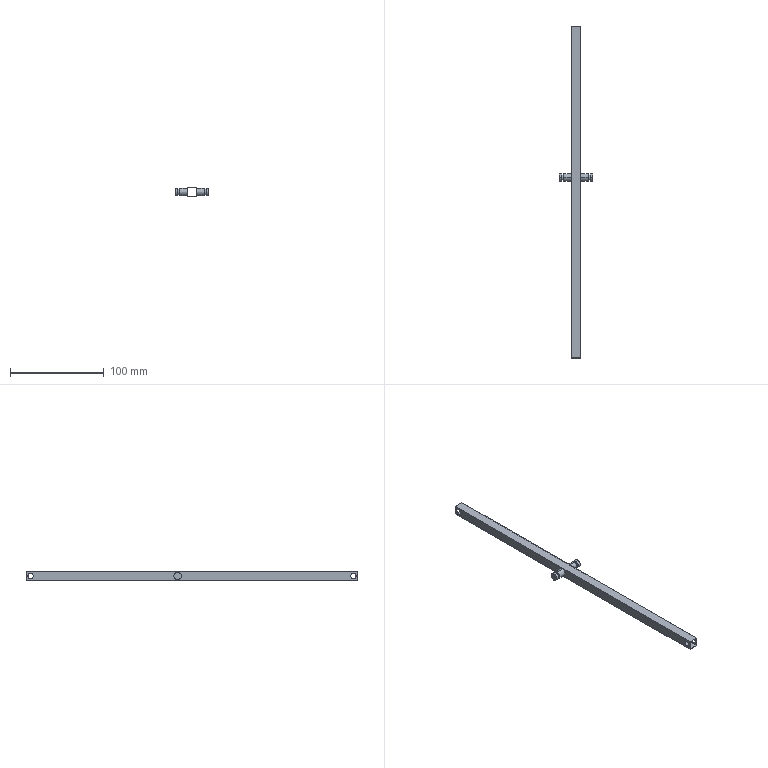Part | SolidWorks | features ICE 5, Extrusion 1, MirrorSolid 1 | 1 solid | 36 faces | box 36 x 355 x 10 mm | volume 7907 mm3 | cylinder 20 | plane 16 | commonest cylinder face diameters 6 x12 8 x8
STEP:
#1=CARTESIAN_POINT('',(-4.5,350.,3.));
#2=VERTEX_POINT('',#1);
#3=CARTESIAN_POINT('',(-4.5,350.,-3.));
#4=VERTEX_POINT('',#3);
#5=CARTESIAN_POINT('',(-4.5,350.,0.));
#6=DIRECTION('',(1.,0.,0.));
#7=DIRECTION('',(0.,0.,-1.));
#8=AXIS2_PLACEMENT_3D('',#5,#6,#7);
#9=CIRCLE('',#8,3.);
#10=EDGE_CURVE('',#2,#4,#9,.T.);
#11=ORIENTED_EDGE('',*,*,#10,.T.);
#12=CARTESIAN_POINT('',(-5.,350.,-3.));
#13=VERTEX_POINT('',#12);
#14=CARTESIAN_POINT('',(13.,350.,-3.));
#15=DIRECTION('',(-1.,0.,0.));
#16=VECTOR('',#15,1000.);
#17=LINE('',#14,#16);
#18=EDGE_CURVE('',#4,#13,#17,.T.);
#19=ORIENTED_EDGE('',*,*,#18,.T.);
#20=CARTESIAN_POINT('',(-5.,350.,3.));
#21=VERTEX_POINT('',#20);
#22=CARTESIAN_POINT('',(-5.,350.,0.));
#23=DIRECTION('',(-1.,0.,0.));
#24=DIRECTION('',(0.,0.,1.));
#25=AXIS2_PLACEMENT_3D('',#22,#23,#24);
#26=CIRCLE('',#25,3.);
#27=EDGE_CURVE('',#13,#21,#26,.T.);
#28=ORIENTED_EDGE('',*,*,#27,.T.);
#29=CARTESIAN_POINT('',(13.,350.,3.));
#30=DIRECTION('',(-1.,0.,0.));
#31=VECTOR('',#30,1000.);
#32=LINE('',#29,#31);
#33=EDGE_CURVE('',#2,#21,#32,.T.);
#34=ORIENTED_EDGE('',*,*,#33,.F.);
#35=EDGE_LOOP('',(#11,#19,#28,#34));
#36=FACE_OUTER_BOUND('',#35,.T.);
#37=CARTESIAN_POINT('',(13.,350.,0.));
#38=DIRECTION('',(-1.,0.,0.));
#39=DIRECTION('',(0.,0.,1.));
#40=AXIS2_PLACEMENT_3D('',#37,#38,#39);
#41=CYLINDRICAL_SURFACE('',#40,3.);
#42=ADVANCED_FACE('',(#36),#41,.F.);
#43=CARTESIAN_POINT('',(5.,350.,-3.));
#44=VERTEX_POINT('',#43);
#45=CARTESIAN_POINT('',(5.,350.,3.));
#46=VERTEX_POINT('',#45);
#47=CARTESIAN_POINT('',(5.,350.,0.));
#48=DIRECTION('',(-1.,0.,0.));
#49=DIRECTION('',(0.,0.,1.));
#50=AXIS2_PLACEMENT_3D('',#47,#48,#49);
#51=CIRCLE('',#50,3.);
#52=EDGE_CURVE('',#44,#46,#51,.T.);
#53=ORIENTED_EDGE('',*,*,#52,.F.);
#54=CARTESIAN_POINT('',(4.5,350.,-3.));
#55=VERTEX_POINT('',#54);
#56=CARTESIAN_POINT('',(13.,350.,-3.));
#57=DIRECTION('',(-1.,0.,0.));
#58=VECTOR('',#57,1000.);
#59=LINE('',#56,#58);
#60=EDGE_CURVE('',#44,#55,#59,.T.);
#61=ORIENTED_EDGE('',*,*,#60,.T.);
#62=CARTESIAN_POINT('',(4.5,350.,3.));
#63=VERTEX_POINT('',#62);
#64=CARTESIAN_POINT('',(4.5,350.,0.));
#65=DIRECTION('',(-1.,0.,0.));
#66=DIRECTION('',(0.,0.,1.));
#67=AXIS2_PLACEMENT_3D('',#64,#65,#66);
#68=CIRCLE('',#67,3.);
#69=EDGE_CURVE('',#55,#63,#68,.T.);
#70=ORIENTED_EDGE('',*,*,#69,.T.);
#71=CARTESIAN_POINT('',(13.,350.,3.));
#72=DIRECTION('',(-1.,0.,0.));
#73=VECTOR('',#72,1000.);
#74=LINE('',#71,#73);
#75=EDGE_CURVE('',#46,#63,#74,.T.);
#76=ORIENTED_EDGE('',*,*,#75,.F.);
#77=EDGE_LOOP('',(#53,#61,#70,#76));
#78=FACE_OUTER_BOUND('',#77,.T.);
#79=CARTESIAN_POINT('',(13.,350.,0.));
#80=DIRECTION('',(-1.,0.,0.));
#81=DIRECTION('',(0.,0.,1.));
#82=AXIS2_PLACEMENT_3D('',#79,#80,#81);
#83=CYLINDRICAL_SURFACE('',#82,3.);
#84=ADVANCED_FACE('',(#78),#83,.F.);
#85=CARTESIAN_POINT('',(-5.,5.,3.));
#86=VERTEX_POINT('',#85);
#87=CARTESIAN_POINT('',(-5.,5.,-3.));
#88=VERTEX_POINT('',#87);
#89=CARTESIAN_POINT('',(-5.,5.,0.));
#90=DIRECTION('',(1.,0.,0.));
#91=DIRECTION('',(0.,0.,-1.));
#92=AXIS2_PLACEMENT_3D('',#89,#90,#91);
#93=CIRCLE('',#92,3.);
#94=EDGE_CURVE('',#86,#88,#93,.T.);
#95=ORIENTED_EDGE('',*,*,#94,.F.);
#96=CARTESIAN_POINT('',(-4.5,5.,3.));
#97=VERTEX_POINT('',#96);
#98=CARTESIAN_POINT('',(-16.,5.,3.));
#99=DIRECTION('',(1.,0.,0.));
#100=VECTOR('',#99,1000.);
#101=LINE('',#98,#100);
#102=EDGE_CURVE('',#86,#97,#101,.T.);
#103=ORIENTED_EDGE('',*,*,#102,.T.);
#104=CARTESIAN_POINT('',(-4.5,5.,-3.));
#105=VERTEX_POINT('',#104);
#106=CARTESIAN_POINT('',(-4.5,5.,0.));
#107=DIRECTION('',(1.,0.,0.));
#108=DIRECTION('',(0.,0.,-1.));
#109=AXIS2_PLACEMENT_3D('',#106,#107,#108);
#110=CIRCLE('',#109,3.);
#111=EDGE_CURVE('',#97,#105,#110,.T.);
#112=ORIENTED_EDGE('',*,*,#111,.T.);
#113=CARTESIAN_POINT('',(-16.,5.,-3.));
#114=DIRECTION('',(1.,0.,0.));
#115=VECTOR('',#114,1000.);
#116=LINE('',#113,#115);
#117=EDGE_CURVE('',#88,#105,#116,.T.);
#118=ORIENTED_EDGE('',*,*,#117,.F.);
#119=EDGE_LOOP('',(#95,#103,#112,#118));
#120=FACE_OUTER_BOUND('',#119,.T.);
#121=CARTESIAN_POINT('',(-16.,5.,0.));
#122=DIRECTION('',(1.,0.,0.));
#123=DIRECTION('',(0.,0.,-1.));
#124=AXIS2_PLACEMENT_3D('',#121,#122,#123);
#125=CYLINDRICAL_SURFACE('',#124,3.);
#126=ADVANCED_FACE('',(#120),#125,.F.);
#127=CARTESIAN_POINT('',(4.5,5.,-3.));
#128=VERTEX_POINT('',#127);
#129=CARTESIAN_POINT('',(4.5,5.,3.));
#130=VERTEX_POINT('',#129);
#131=CARTESIAN_POINT('',(4.5,5.,0.));
#132=DIRECTION('',(-1.,0.,0.));
#133=DIRECTION('',(0.,0.,1.));
#134=AXIS2_PLACEMENT_3D('',#131,#132,#133);
#135=CIRCLE('',#134,3.);
#136=EDGE_CURVE('',#128,#130,#135,.T.);
#137=ORIENTED_EDGE('',*,*,#136,.T.);
#138=CARTESIAN_POINT('',(5.,5.,3.));
#139=VERTEX_POINT('',#138);
#140=CARTESIAN_POINT('',(-16.,5.,3.));
#141=DIRECTION('',(1.,0.,0.));
#142=VECTOR('',#141,1000.);
#143=LINE('',#140,#142);
#144=EDGE_CURVE('',#130,#139,#143,.T.);
#145=ORIENTED_EDGE('',*,*,#144,.T.);
#146=CARTESIAN_POINT('',(5.,5.,-3.));
#147=VERTEX_POINT('',#146);
#148=CARTESIAN_POINT('',(5.,5.,0.));
#149=DIRECTION('',(1.,0.,0.));
#150=DIRECTION('',(0.,0.,-1.));
#151=AXIS2_PLACEMENT_3D('',#148,#149,#150);
#152=CIRCLE('',#151,3.);
#153=EDGE_CURVE('',#139,#147,#152,.T.);
#154=ORIENTED_EDGE('',*,*,#153,.T.);
#155=CARTESIAN_POINT('',(-16.,5.,-3.));
#156=DIRECTION('',(1.,0.,0.));
#157=VECTOR('',#156,1000.);
#158=LINE('',#155,#157);
#159=EDGE_CURVE('',#128,#147,#158,.T.);
#160=ORIENTED_EDGE('',*,*,#159,.F.);
#161=EDGE_LOOP('',(#137,#145,#154,#160));
#162=FACE_OUTER_BOUND('',#161,.T.);
#163=CARTESIAN_POINT('',(-16.,5.,0.));
#164=DIRECTION('',(1.,0.,0.));
#165=DIRECTION('',(0.,0.,-1.));
#166=AXIS2_PLACEMENT_3D('',#163,#164,#165);
#167=CYLINDRICAL_SURFACE('',#166,3.);
#168=ADVANCED_FACE('',(#162),#167,.F.);
#169=CARTESIAN_POINT('',(-18.,193.,4.));
#170=VERTEX_POINT('',#169);
#171=CARTESIAN_POINT('',(-18.,193.,-4.));
#172=VERTEX_POINT('',#171);
#173=CARTESIAN_POINT('',(-18.,193.,0.));
#174=DIRECTION('',(1.,0.,0.));
#175=DIRECTION('',(0.,0.,-1.));
#176=AXIS2_PLACEMENT_3D('',#173,#174,#175);
#177=CIRCLE('',#176,4.);
#178=EDGE_CURVE('',#170,#172,#177,.T.);
#179=ORIENTED_EDGE('',*,*,#178,.T.);
#180=CARTESIAN_POINT('',(-15.,193.,-4.));
#181=VERTEX_POINT('',#180);
#182=CARTESIAN_POINT('',(-18.,193.,-4.));
#183=DIRECTION('',(1.,0.,0.));
#184=VECTOR('',#183,1000.);
#185=LINE('',#182,#184);
#186=EDGE_CURVE('',#172,#181,#185,.T.);
#187=ORIENTED_EDGE('',*,*,#186,.T.);
#188=CARTESIAN_POINT('',(-15.,193.,4.));
#189=VERTEX_POINT('',#188);
#190=CARTESIAN_POINT('',(-15.,193.,0.));
#191=DIRECTION('',(1.,0.,0.));
#192=DIRECTION('',(0.,0.,-1.));
#193=AXIS2_PLACEMENT_3D('',#190,#191,#192);
#194=CIRCLE('',#193,4.);
#195=EDGE_CURVE('',#189,#181,#194,.T.);
#196=ORIENTED_EDGE('',*,*,#195,.F.);
#197=CARTESIAN_POINT('',(-18.,193.,4.));
#198=DIRECTION('',(1.,0.,0.));
#199=VECTOR('',#198,1000.);
#200=LINE('',#197,#199);
#201=EDGE_CURVE('',#170,#189,#200,.T.);
#202=ORIENTED_EDGE('',*,*,#201,.F.);
#203=EDGE_LOOP('',(#179,#187,#196,#202));
#204=FACE_OUTER_BOUND('',#203,.T.);
#205=CARTESIAN_POINT('',(-18.,193.,0.));
#206=DIRECTION('',(1.,0.,0.));
#207=DIRECTION('',(0.,0.,1.));
#208=AXIS2_PLACEMENT_3D('',#205,#206,#207);
#209=CYLINDRICAL_SURFACE('',#208,4.);
#210=ADVANCED_FACE('',(#204),#209,.T.);
#211=CARTESIAN_POINT('',(-15.,193.,3.));
#212=VERTEX_POINT('',#211);
#213=CARTESIAN_POINT('',(-15.,193.,-3.));
#214=VERTEX_POINT('',#213);
#215=CARTESIAN_POINT('',(-15.,193.,0.));
#216=DIRECTION('',(1.,0.,0.));
#217=DIRECTION('',(0.,0.,-1.));
#218=AXIS2_PLACEMENT_3D('',#215,#216,#217);
#219=CIRCLE('',#218,3.);
#220=EDGE_CURVE('',#212,#214,#219,.T.);
#221=ORIENTED_EDGE('',*,*,#220,.T.);
#222=CARTESIAN_POINT('',(-13.,193.,-3.));
#223=VERTEX_POINT('',#222);
#224=CARTESIAN_POINT('',(-15.,193.,-3.));
#225=DIRECTION('',(1.,0.,0.));
#226=VECTOR('',#225,1000.);
#227=LINE('',#224,#226);
#228=EDGE_CURVE('',#214,#223,#227,.T.);
#229=ORIENTED_EDGE('',*,*,#228,.T.);
#230=CARTESIAN_POINT('',(-13.,193.,3.));
#231=VERTEX_POINT('',#230);
#232=CARTESIAN_POINT('',(-13.,193.,0.));
#233=DIRECTION('',(1.,0.,0.));
#234=DIRECTION('',(0.,0.,-1.));
#235=AXIS2_PLACEMENT_3D('',#232,#233,#234);
#236=CIRCLE('',#235,3.);
#237=EDGE_CURVE('',#231,#223,#236,.T.);
#238=ORIENTED_EDGE('',*,*,#237,.F.);
#239=CARTESIAN_POINT('',(-15.,193.,3.));
#240=DIRECTION('',(1.,0.,0.));
#241=VECTOR('',#240,1000.);
#242=LINE('',#239,#241);
#243=EDGE_CURVE('',#212,#231,#242,.T.);
#244=ORIENTED_EDGE('',*,*,#243,.F.);
#245=EDGE_LOOP('',(#221,#229,#238,#244));
#246=FACE_OUTER_BOUND('',#245,.T.);
#247=CARTESIAN_POINT('',(-15.,193.,0.));
#248=DIRECTION('',(1.,0.,0.));
#249=DIRECTION('',(0.,0.,1.));
#250=AXIS2_PLACEMENT_3D('',#247,#248,#249);
#251=CYLINDRICAL_SURFACE('',#250,3.);
#252=ADVANCED_FACE('',(#246),#251,.T.);
#253=CARTESIAN_POINT('',(-13.,193.,4.));
#254=VERTEX_POINT('',#253);
#255=CARTESIAN_POINT('',(-13.,193.,-4.));
#256=VERTEX_POINT('',#255);
#257=CARTESIAN_POINT('',(-13.,193.,0.));
#258=DIRECTION('',(1.,0.,0.));
#259=DIRECTION('',(0.,0.,-1.));
#260=AXIS2_PLACEMENT_3D('',#257,#258,#259);
#261=CIRCLE('',#260,4.);
#262=EDGE_CURVE('',#254,#256,#261,.T.);
#263=ORIENTED_EDGE('',*,*,#262,.T.);
#264=CARTESIAN_POINT('',(-5.,193.,-4.));
#265=VERTEX_POINT('',#264);
#266=CARTESIAN_POINT('',(-13.,193.,-4.));
#267=DIRECTION('',(1.,0.,0.));
#268=VECTOR('',#267,1000.);
#269=LINE('',#266,#268);
#270=EDGE_CURVE('',#256,#265,#269,.T.);
#271=ORIENTED_EDGE('',*,*,#270,.T.);
#272=CARTESIAN_POINT('',(-5.,193.,4.));
#273=VERTEX_POINT('',#272);
#274=CARTESIAN_POINT('',(-5.,193.,0.));
#275=DIRECTION('',(-1.,0.,0.));
#276=DIRECTION('',(0.,0.,-1.));
#277=AXIS2_PLACEMENT_3D('',#274,#275,#276);
#278=CIRCLE('',#277,4.);
#279=EDGE_CURVE('',#265,#273,#278,.T.);
#280=ORIENTED_EDGE('',*,*,#279,.T.);
#281=CARTESIAN_POINT('',(-13.,193.,4.));
#282=DIRECTION('',(1.,0.,0.));
#283=VECTOR('',#282,1000.);
#284=LINE('',#281,#283);
#285=EDGE_CURVE('',#254,#273,#284,.T.);
#286=ORIENTED_EDGE('',*,*,#285,.F.);
#287=EDGE_LOOP('',(#263,#271,#280,#286));
#288=FACE_OUTER_BOUND('',#287,.T.);
#289=CARTESIAN_POINT('',(-13.,193.,0.));
#290=DIRECTION('',(1.,0.,0.));
#291=DIRECTION('',(0.,0.,1.));
#292=AXIS2_PLACEMENT_3D('',#289,#290,#291);
#293=CYLINDRICAL_SURFACE('',#292,4.);
#294=ADVANCED_FACE('',(#288),#293,.T.);
#295=CARTESIAN_POINT('',(18.,193.,-4.));
#296=VERTEX_POINT('',#295);
#297=CARTESIAN_POINT('',(18.,193.,4.));
#298=VERTEX_POINT('',#297);
#299=CARTESIAN_POINT('',(18.,193.,0.));
#300=DIRECTION('',(1.,0.,0.));
#301=DIRECTION('',(0.,0.,-1.));
#302=AXIS2_PLACEMENT_3D('',#299,#300,#301);
#303=CIRCLE('',#302,4.);
#304=EDGE_CURVE('',#296,#298,#303,.T.);
#305=ORIENTED_EDGE('',*,*,#304,.F.);
#306=CARTESIAN_POINT('',(15.,193.,-4.));
#307=VERTEX_POINT('',#306);
#308=CARTESIAN_POINT('',(18.,193.,-4.));
#309=DIRECTION('',(-1.,0.,0.));
#310=VECTOR('',#309,1000.);
#311=LINE('',#308,#310);
#312=EDGE_CURVE('',#296,#307,#311,.T.);
#313=ORIENTED_EDGE('',*,*,#312,.T.);
#314=CARTESIAN_POINT('',(15.,193.,4.));
#315=VERTEX_POINT('',#314);
#316=CARTESIAN_POINT('',(15.,193.,0.));
#317=DIRECTION('',(1.,0.,0.));
#318=DIRECTION('',(0.,0.,-1.));
#319=AXIS2_PLACEMENT_3D('',#316,#317,#318);
#320=CIRCLE('',#319,4.);
#321=EDGE_CURVE('',#307,#315,#320,.T.);
#322=ORIENTED_EDGE('',*,*,#321,.T.);
#323=CARTESIAN_POINT('',(18.,193.,4.));
#324=DIRECTION('',(-1.,0.,0.));
#325=VECTOR('',#324,1000.);
#326=LINE('',#323,#325);
#327=EDGE_CURVE('',#298,#315,#326,.T.);
#328=ORIENTED_EDGE('',*,*,#327,.F.);
#329=EDGE_LOOP('',(#305,#313,#322,#328));
#330=FACE_OUTER_BOUND('',#329,.T.);
#331=CARTESIAN_POINT('',(18.,193.,0.));
#332=DIRECTION('',(-1.,0.,0.));
#333=DIRECTION('',(0.,0.,1.));
#334=AXIS2_PLACEMENT_3D('',#331,#332,#333);
#335=CYLINDRICAL_SURFACE('',#334,4.);
#336=ADVANCED_FACE('',(#330),#335,.T.);
#337=CARTESIAN_POINT('',(15.,193.,-3.));
#338=VERTEX_POINT('',#337);
#339=CARTESIAN_POINT('',(15.,193.,3.));
#340=VERTEX_POINT('',#339);
#341=CARTESIAN_POINT('',(15.,193.,0.));
#342=DIRECTION('',(1.,0.,0.));
#343=DIRECTION('',(0.,0.,-1.));
#344=AXIS2_PLACEMENT_3D('',#341,#342,#343);
#345=CIRCLE('',#344,3.);
#346=EDGE_CURVE('',#338,#340,#345,.T.);
#347=ORIENTED_EDGE('',*,*,#346,.F.);
#348=CARTESIAN_POINT('',(13.,193.,-3.));
#349=VERTEX_POINT('',#348);
#350=CARTESIAN_POINT('',(15.,193.,-3.));
#351=DIRECTION('',(-1.,0.,0.));
#352=VECTOR('',#351,1000.);
#353=LINE('',#350,#352);
#354=EDGE_CURVE('',#338,#349,#353,.T.);
#355=ORIENTED_EDGE('',*,*,#354,.T.);
#356=CARTESIAN_POINT('',(13.,193.,3.));
#357=VERTEX_POINT('',#356);
#358=CARTESIAN_POINT('',(13.,193.,0.));
#359=DIRECTION('',(1.,0.,0.));
#360=DIRECTION('',(0.,0.,-1.));
#361=AXIS2_PLACEMENT_3D('',#358,#359,#360);
#362=CIRCLE('',#361,3.);
#363=EDGE_CURVE('',#349,#357,#362,.T.);
#364=ORIENTED_EDGE('',*,*,#363,.T.);
#365=CARTESIAN_POINT('',(15.,193.,3.));
#366=DIRECTION('',(-1.,0.,0.));
#367=VECTOR('',#366,1000.);
#368=LINE('',#365,#367);
#369=EDGE_CURVE('',#340,#357,#368,.T.);
#370=ORIENTED_EDGE('',*,*,#369,.F.);
#371=EDGE_LOOP('',(#347,#355,#364,#370));
#372=FACE_OUTER_BOUND('',#371,.T.);
#373=CARTESIAN_POINT('',(15.,193.,0.));
#374=DIRECTION('',(-1.,0.,0.));
#375=DIRECTION('',(0.,0.,1.));
#376=AXIS2_PLACEMENT_3D('',#373,#374,#375);
#377=CYLINDRICAL_SURFACE('',#376,3.);
#378=ADVANCED_FACE('',(#372),#377,.T.);
#379=CARTESIAN_POINT('',(13.,193.,-4.));
#380=VERTEX_POINT('',#379);
#381=CARTESIAN_POINT('',(13.,193.,4.));
#382=VERTEX_POINT('',#381);
#383=CARTESIAN_POINT('',(13.,193.,0.));
#384=DIRECTION('',(1.,0.,0.));
#385=DIRECTION('',(0.,0.,-1.));
#386=AXIS2_PLACEMENT_3D('',#383,#384,#385);
#387=CIRCLE('',#386,4.);
#388=EDGE_CURVE('',#380,#382,#387,.T.);
#389=ORIENTED_EDGE('',*,*,#388,.F.);
#390=CARTESIAN_POINT('',(5.,193.,-4.));
#391=VERTEX_POINT('',#390);
#392=CARTESIAN_POINT('',(13.,193.,-4.));
#393=DIRECTION('',(-1.,0.,0.));
#394=VECTOR('',#393,1000.);
#395=LINE('',#392,#394);
#396=EDGE_CURVE('',#380,#391,#395,.T.);
#397=ORIENTED_EDGE('',*,*,#396,.T.);
#398=CARTESIAN_POINT('',(5.,193.,4.));
#399=VERTEX_POINT('',#398);
#400=CARTESIAN_POINT('',(5.,193.,0.));
#401=DIRECTION('',(1.,0.,0.));
#402=DIRECTION('',(0.,0.,1.));
#403=AXIS2_PLACEMENT_3D('',#400,#401,#402);
#404=CIRCLE('',#403,4.);
#405=EDGE_CURVE('',#391,#399,#404,.T.);
#406=ORIENTED_EDGE('',*,*,#405,.T.);
#407=CARTESIAN_POINT('',(13.,193.,4.));
#408=DIRECTION('',(-1.,0.,0.));
#409=VECTOR('',#408,1000.);
#410=LINE('',#407,#409);
#411=EDGE_CURVE('',#382,#399,#410,.T.);
#412=ORIENTED_EDGE('',*,*,#411,.F.);
#413=EDGE_LOOP('',(#389,#397,#406,#412));
#414=FACE_OUTER_BOUND('',#413,.T.);
#415=CARTESIAN_POINT('',(13.,193.,0.));
#416=DIRECTION('',(-1.,0.,0.));
#417=DIRECTION('',(0.,0.,1.));
#418=AXIS2_PLACEMENT_3D('',#415,#416,#417);
#419=CYLINDRICAL_SURFACE('',#418,4.);
#420=ADVANCED_FACE('',(#414),#419,.T.);
#421=CARTESIAN_POINT('',(5.,355.,5.));
#422=VERTEX_POINT('',#421);
#423=CARTESIAN_POINT('',(5.,355.,-5.));
#424=VERTEX_POINT('',#423);
#425=CARTESIAN_POINT('',(5.,355.,-5.));
#426=DIRECTION('',(0.,0.,-1.));
#427=VECTOR('',#426,1000.);
#428=LINE('',#425,#427);
#429=EDGE_CURVE('',#422,#424,#428,.T.);
#430=ORIENTED_EDGE('',*,*,#429,.T.);
#431=CARTESIAN_POINT('',(-5.,355.,-5.));
#432=VERTEX_POINT('',#431);
#433=CARTESIAN_POINT('',(-5.,355.,-5.));
#434=DIRECTION('',(-1.,0.,0.));
#435=VECTOR('',#434,1000.);
#436=LINE('',#433,#435);
#437=EDGE_CURVE('',#424,#432,#436,.T.);
#438=ORIENTED_EDGE('',*,*,#437,.T.);
#439=CARTESIAN_POINT('',(-5.,355.,5.));
#440=VERTEX_POINT('',#439);
#441=CARTESIAN_POINT('',(-5.,355.,-5.));
#442=DIRECTION('',(0.,0.,1.));
#443=VECTOR('',#442,1000.);
#444=LINE('',#441,#443);
#445=EDGE_CURVE('',#432,#440,#444,.T.);
#446=ORIENTED_EDGE('',*,*,#445,.T.);
#447=CARTESIAN_POINT('',(-5.,355.,5.));
#448=DIRECTION('',(1.,0.,0.));
#449=VECTOR('',#448,1000.);
#450=LINE('',#447,#449);
#451=EDGE_CURVE('',#440,#422,#450,.T.);
#452=ORIENTED_EDGE('',*,*,#451,.T.);
#453=EDGE_LOOP('',(#430,#438,#446,#452));
#454=FACE_OUTER_BOUND('',#453,.T.);
#455=CARTESIAN_POINT('',(-4.5,355.,-4.5));
#456=VERTEX_POINT('',#455);
#457=CARTESIAN_POINT('',(-4.5,355.,4.5));
#458=VERTEX_POINT('',#457);
#459=CARTESIAN_POINT('',(-4.5,355.,-4.5));
#460=DIRECTION('',(0.,0.,1.));
#461=VECTOR('',#460,1000.);
#462=LINE('',#459,#461);
#463=EDGE_CURVE('',#456,#458,#462,.T.);
#464=ORIENTED_EDGE('',*,*,#463,.F.);
#465=CARTESIAN_POINT('',(4.5,355.,-4.5));
#466=VERTEX_POINT('',#465);
#467=CARTESIAN_POINT('',(-4.5,355.,-4.5));
#468=DIRECTION('',(-1.,0.,0.));
#469=VECTOR('',#468,1000.);
#470=LINE('',#467,#469);
#471=EDGE_CURVE('',#466,#456,#470,.T.);
#472=ORIENTED_EDGE('',*,*,#471,.F.);
#473=CARTESIAN_POINT('',(4.5,355.,4.5));
#474=VERTEX_POINT('',#473);
#475=CARTESIAN_POINT('',(4.5,355.,-4.5));
#476=DIRECTION('',(0.,0.,-1.));
#477=VECTOR('',#476,1000.);
#478=LINE('',#475,#477);
#479=EDGE_CURVE('',#474,#466,#478,.T.);
#480=ORIENTED_EDGE('',*,*,#479,.F.);
#481=CARTESIAN_POINT('',(-4.5,355.,4.5));
#482=DIRECTION('',(1.,0.,0.));
#483=VECTOR('',#482,1000.);
#484=LINE('',#481,#483);
#485=EDGE_CURVE('',#458,#474,#484,.T.);
#486=ORIENTED_EDGE('',*,*,#485,.F.);
#487=EDGE_LOOP('',(#464,#472,#480,#486));
#488=FACE_BOUND('',#487,.T.);
#489=CARTESIAN_POINT('',(0.,355.,0.));
#490=DIRECTION('',(0.,1.,0.));
#491=DIRECTION('',(0.,0.,1.));
#492=AXIS2_PLACEMENT_3D('',#489,#490,#491);
#493=PLANE('',#492);
#494=ADVANCED_FACE('',(#454,#488),#493,.T.);
#495=CARTESIAN_POINT('',(5.,0.,5.));
#496=VERTEX_POINT('',#495);
#497=CARTESIAN_POINT('',(5.,0.,-5.));
#498=VERTEX_POINT('',#497);
#499=CARTESIAN_POINT('',(5.,0.,-5.));
#500=DIRECTION('',(0.,0.,-1.));
#501=VECTOR('',#500,1000.);
#502=LINE('',#499,#501);
#503=EDGE_CURVE('',#496,#498,#502,.T.);
#504=ORIENTED_EDGE('',*,*,#503,.F.);
#505=CARTESIAN_POINT('',(-5.,0.,5.));
#506=VERTEX_POINT('',#505);
#507=CARTESIAN_POINT('',(-5.,0.,5.));
#508=DIRECTION('',(1.,0.,0.));
#509=VECTOR('',#508,1000.);
#510=LINE('',#507,#509);
#511=EDGE_CURVE('',#506,#496,#510,.T.);
#512=ORIENTED_EDGE('',*,*,#511,.F.);
#513=CARTESIAN_POINT('',(-5.,0.,-5.));
#514=VERTEX_POINT('',#513);
#515=CARTESIAN_POINT('',(-5.,0.,-5.));
#516=DIRECTION('',(0.,0.,1.));
#517=VECTOR('',#516,1000.);
#518=LINE('',#515,#517);
#519=EDGE_CURVE('',#514,#506,#518,.T.);
#520=ORIENTED_EDGE('',*,*,#519,.F.);
#521=CARTESIAN_POINT('',(-5.,0.,-5.));
#522=DIRECTION('',(-1.,0.,0.));
#523=VECTOR('',#522,1000.);
#524=LINE('',#521,#523);
#525=EDGE_CURVE('',#498,#514,#524,.T.);
#526=ORIENTED_EDGE('',*,*,#525,.F.);
#527=EDGE_LOOP('',(#504,#512,#520,#526));
#528=FACE_OUTER_BOUND('',#527,.T.);
#529=CARTESIAN_POINT('',(4.5,0.,-4.5));
#530=VERTEX_POINT('',#529);
#531=CARTESIAN_POINT('',(-4.5,0.,-4.5));
#532=VERTEX_POINT('',#531);
#533=CARTESIAN_POINT('',(-4.5,0.,-4.5));
#534=DIRECTION('',(-1.,0.,0.));
#535=VECTOR('',#534,1000.);
#536=LINE('',#533,#535);
#537=EDGE_CURVE('',#530,#532,#536,.T.);
#538=ORIENTED_EDGE('',*,*,#537,.T.);
#539=CARTESIAN_POINT('',(-4.5,0.,4.5));
#540=VERTEX_POINT('',#539);
#541=CARTESIAN_POINT('',(-4.5,0.,-4.5));
#542=DIRECTION('',(0.,0.,1.));
#543=VECTOR('',#542,1000.);
#544=LINE('',#541,#543);
#545=EDGE_CURVE('',#532,#540,#544,.T.);
#546=ORIENTED_EDGE('',*,*,#545,.T.);
#547=CARTESIAN_POINT('',(4.5,0.,4.5));
#548=VERTEX_POINT('',#547);
#549=CARTESIAN_POINT('',(-4.5,0.,4.5));
#550=DIRECTION('',(1.,0.,0.));
#551=VECTOR('',#550,1000.);
#552=LINE('',#549,#551);
#553=EDGE_CURVE('',#540,#548,#552,.T.);
#554=ORIENTED_EDGE('',*,*,#553,.T.);
#555=CARTESIAN_POINT('',(4.5,0.,-4.5));
#556=DIRECTION('',(0.,0.,-1.));
#557=VECTOR('',#556,1000.);
#558=LINE('',#555,#557);
#559=EDGE_CURVE('',#548,#530,#558,.T.);
#560=ORIENTED_EDGE('',*,*,#559,.T.);
#561=EDGE_LOOP('',(#538,#546,#554,#560));
#562=FACE_BOUND('',#561,.T.);
#563=CARTESIAN_POINT('',(0.,0.,0.));
#564=DIRECTION('',(0.,1.,0.));
#565=DIRECTION('',(0.,0.,1.));
#566=AXIS2_PLACEMENT_3D('',#563,#564,#565);
#567=PLANE('',#566);
#568=ADVANCED_FACE('',(#528,#562),#567,.F.);
#569=CARTESIAN_POINT('',(5.,350.,0.));
#570=DIRECTION('',(-1.,0.,0.));
#571=DIRECTION('',(0.,0.,1.));
#572=AXIS2_PLACEMENT_3D('',#569,#570,#571);
#573=CIRCLE('',#572,3.);
#574=EDGE_CURVE('',#46,#44,#573,.T.);
#575=ORIENTED_EDGE('',*,*,#574,.T.);
#576=ORIENTED_EDGE('',*,*,#52,.T.);
#577=EDGE_LOOP('',(#575,#576));
#578=FACE_BOUND('',#577,.T.);
#579=CARTESIAN_POINT('',(5.,5.,0.));
#580=DIRECTION('',(1.,0.,0.));
#581=DIRECTION('',(0.,0.,-1.));
#582=AXIS2_PLACEMENT_3D('',#579,#580,#581);
#583=CIRCLE('',#582,3.);
#584=EDGE_CURVE('',#147,#139,#583,.T.);
#585=ORIENTED_EDGE('',*,*,#584,.F.);
#586=ORIENTED_EDGE('',*,*,#153,.F.);
#587=EDGE_LOOP('',(#585,#586));
#588=FACE_BOUND('',#587,.T.);
#589=CARTESIAN_POINT('',(5.,193.,0.));
#590=DIRECTION('',(1.,0.,0.));
#591=DIRECTION('',(0.,0.,1.));
#592=AXIS2_PLACEMENT_3D('',#589,#590,#591);
#593=CIRCLE('',#592,4.);
#594=EDGE_CURVE('',#399,#391,#593,.T.);
#595=ORIENTED_EDGE('',*,*,#594,.F.);
#596=ORIENTED_EDGE('',*,*,#405,.F.);
#597=EDGE_LOOP('',(#595,#596));
#598=FACE_BOUND('',#597,.T.);
#599=ORIENTED_EDGE('',*,*,#503,.T.);
#600=CARTESIAN_POINT('',(5.,355.,-5.));
#601=DIRECTION('',(0.,-1.,0.));
#602=VECTOR('',#601,1000.);
#603=LINE('',#600,#602);
#604=EDGE_CURVE('',#424,#498,#603,.T.);
#605=ORIENTED_EDGE('',*,*,#604,.F.);
#606=ORIENTED_EDGE('',*,*,#429,.F.);
#607=CARTESIAN_POINT('',(5.,355.,5.));
#608=DIRECTION('',(0.,-1.,0.));
#609=VECTOR('',#608,1000.);
#610=LINE('',#607,#609);
#611=EDGE_CURVE('',#422,#496,#610,.T.);
#612=ORIENTED_EDGE('',*,*,#611,.T.);
#613=EDGE_LOOP('',(#599,#605,#606,#612));
#614=FACE_OUTER_BOUND('',#613,.T.);
#615=CARTESIAN_POINT('',(5.,355.,-5.));
#616=DIRECTION('',(-1.,0.,0.));
#617=DIRECTION('',(0.,0.,1.));
#618=AXIS2_PLACEMENT_3D('',#615,#616,#617);
#619=PLANE('',#618);
#620=ADVANCED_FACE('',(#578,#588,#598,#614),#619,.F.);
#621=ORIENTED_EDGE('',*,*,#525,.T.);
#622=CARTESIAN_POINT('',(-5.,355.,-5.));
#623=DIRECTION('',(0.,-1.,0.));
#624=VECTOR('',#623,1000.);
#625=LINE('',#622,#624);
#626=EDGE_CURVE('',#432,#514,#625,.T.);
#627=ORIENTED_EDGE('',*,*,#626,.F.);
#628=ORIENTED_EDGE('',*,*,#437,.F.);
#629=ORIENTED_EDGE('',*,*,#604,.T.);
#630=EDGE_LOOP('',(#621,#627,#628,#629));
#631=FACE_OUTER_BOUND('',#630,.T.);
#632=CARTESIAN_POINT('',(-5.,355.,-5.));
#633=DIRECTION('',(0.,0.,1.));
#634=DIRECTION('',(1.,0.,0.));
#635=AXIS2_PLACEMENT_3D('',#632,#633,#634);
#636=PLANE('',#635);
#637=ADVANCED_FACE('',(#631),#636,.F.);
#638=CARTESIAN_POINT('',(-5.,350.,0.));
#639=DIRECTION('',(-1.,0.,0.));
#640=DIRECTION('',(0.,0.,1.));
#641=AXIS2_PLACEMENT_3D('',#638,#639,#640);
#642=CIRCLE('',#641,3.);
#643=EDGE_CURVE('',#21,#13,#642,.T.);
#644=ORIENTED_EDGE('',*,*,#643,.F.);
#645=ORIENTED_EDGE('',*,*,#27,.F.);
#646=EDGE_LOOP('',(#644,#645));
#647=FACE_BOUND('',#646,.T.);
#648=CARTESIAN_POINT('',(-5.,5.,0.));
#649=DIRECTION('',(1.,0.,0.));
#650=DIRECTION('',(0.,0.,-1.));
#651=AXIS2_PLACEMENT_3D('',#648,#649,#650);
#652=CIRCLE('',#651,3.);
#653=EDGE_CURVE('',#88,#86,#652,.T.);
#654=ORIENTED_EDGE('',*,*,#653,.T.);
#655=ORIENTED_EDGE('',*,*,#94,.T.);
#656=EDGE_LOOP('',(#654,#655));
#657=FACE_BOUND('',#656,.T.);
#658=CARTESIAN_POINT('',(-5.,193.,0.));
#659=DIRECTION('',(-1.,0.,0.));
#660=DIRECTION('',(0.,0.,-1.));
#661=AXIS2_PLACEMENT_3D('',#658,#659,#660);
#662=CIRCLE('',#661,4.);
#663=EDGE_CURVE('',#273,#265,#662,.T.);
#664=ORIENTED_EDGE('',*,*,#663,.F.);
#665=ORIENTED_EDGE('',*,*,#279,.F.);
#666=EDGE_LOOP('',(#664,#665));
#667=FACE_BOUND('',#666,.T.);
#668=ORIENTED_EDGE('',*,*,#519,.T.);
#669=CARTESIAN_POINT('',(-5.,355.,5.));
#670=DIRECTION('',(0.,-1.,0.));
#671=VECTOR('',#670,1000.);
#672=LINE('',#669,#671);
#673=EDGE_CURVE('',#440,#506,#672,.T.);
#674=ORIENTED_EDGE('',*,*,#673,.F.);
#675=ORIENTED_EDGE('',*,*,#445,.F.);
#676=ORIENTED_EDGE('',*,*,#626,.T.);
#677=EDGE_LOOP('',(#668,#674,#675,#676));
#678=FACE_OUTER_BOUND('',#677,.T.);
#679=CARTESIAN_POINT('',(-5.,355.,-5.));
#680=DIRECTION('',(1.,0.,0.));
#681=DIRECTION('',(0.,0.,-1.));
#682=AXIS2_PLACEMENT_3D('',#679,#680,#681);
#683=PLANE('',#682);
#684=ADVANCED_FACE('',(#647,#657,#667,#678),#683,.F.);
#685=ORIENTED_EDGE('',*,*,#511,.T.);
#686=ORIENTED_EDGE('',*,*,#611,.F.);
#687=ORIENTED_EDGE('',*,*,#451,.F.);
#688=ORIENTED_EDGE('',*,*,#673,.T.);
#689=EDGE_LOOP('',(#685,#686,#687,#688));
#690=FACE_OUTER_BOUND('',#689,.T.);
#691=CARTESIAN_POINT('',(-5.,355.,5.));
#692=DIRECTION('',(0.,0.,-1.));
#693=DIRECTION('',(-1.,0.,0.));
#694=AXIS2_PLACEMENT_3D('',#691,#692,#693);
#695=PLANE('',#694);
#696=ADVANCED_FACE('',(#690),#695,.F.);
#697=ORIENTED_EDGE('',*,*,#537,.F.);
#698=CARTESIAN_POINT('',(4.5,355.,-4.5));
#699=DIRECTION('',(0.,-1.,0.));
#700=VECTOR('',#699,1000.);
#701=LINE('',#698,#700);
#702=EDGE_CURVE('',#466,#530,#701,.T.);
#703=ORIENTED_EDGE('',*,*,#702,.F.);
#704=ORIENTED_EDGE('',*,*,#471,.T.);
#705=CARTESIAN_POINT('',(-4.5,355.,-4.5));
#706=DIRECTION('',(0.,-1.,0.));
#707=VECTOR('',#706,1000.);
#708=LINE('',#705,#707);
#709=EDGE_CURVE('',#456,#532,#708,.T.);
#710=ORIENTED_EDGE('',*,*,#709,.T.);
#711=EDGE_LOOP('',(#697,#703,#704,#710));
#712=FACE_OUTER_BOUND('',#711,.T.);
#713=CARTESIAN_POINT('',(-4.5,355.,-4.5));
#714=DIRECTION('',(0.,0.,1.));
#715=DIRECTION('',(1.,0.,0.));
#716=AXIS2_PLACEMENT_3D('',#713,#714,#715);
#717=PLANE('',#716);
#718=ADVANCED_FACE('',(#712),#717,.T.);
#719=ORIENTED_EDGE('',*,*,#10,.F.);
#720=CARTESIAN_POINT('',(-4.5,350.,0.));
#721=DIRECTION('',(1.,0.,0.));
#722=DIRECTION('',(0.,0.,-1.));
#723=AXIS2_PLACEMENT_3D('',#720,#721,#722);
#724=CIRCLE('',#723,3.);
#725=EDGE_CURVE('',#4,#2,#724,.T.);
#726=ORIENTED_EDGE('',*,*,#725,.F.);
#727=EDGE_LOOP('',(#719,#726));
#728=FACE_BOUND('',#727,.T.);
#729=CARTESIAN_POINT('',(-4.5,5.,0.));
#730=DIRECTION('',(1.,0.,0.));
#731=DIRECTION('',(0.,0.,-1.));
#732=AXIS2_PLACEMENT_3D('',#729,#730,#731);
#733=CIRCLE('',#732,3.);
#734=EDGE_CURVE('',#105,#97,#733,.T.);
#735=ORIENTED_EDGE('',*,*,#734,.F.);
#736=ORIENTED_EDGE('',*,*,#111,.F.);
#737=EDGE_LOOP('',(#735,#736));
#738=FACE_BOUND('',#737,.T.);
#739=ORIENTED_EDGE('',*,*,#545,.F.);
#740=ORIENTED_EDGE('',*,*,#709,.F.);
#741=ORIENTED_EDGE('',*,*,#463,.T.);
#742=CARTESIAN_POINT('',(-4.5,355.,4.5));
#743=DIRECTION('',(0.,-1.,0.));
#744=VECTOR('',#743,1000.);
#745=LINE('',#742,#744);
#746=EDGE_CURVE('',#458,#540,#745,.T.);
#747=ORIENTED_EDGE('',*,*,#746,.T.);
#748=EDGE_LOOP('',(#739,#740,#741,#747));
#749=FACE_OUTER_BOUND('',#748,.T.);
#750=CARTESIAN_POINT('',(-4.5,355.,-4.5));
#751=DIRECTION('',(1.,0.,0.));
#752=DIRECTION('',(0.,0.,-1.));
#753=AXIS2_PLACEMENT_3D('',#750,#751,#752);
#754=PLANE('',#753);
#755=ADVANCED_FACE('',(#728,#738,#749),#754,.T.);
#756=ORIENTED_EDGE('',*,*,#553,.F.);
#757=ORIENTED_EDGE('',*,*,#746,.F.);
#758=ORIENTED_EDGE('',*,*,#485,.T.);
#759=CARTESIAN_POINT('',(4.5,355.,4.5));
#760=DIRECTION('',(0.,-1.,0.));
#761=VECTOR('',#760,1000.);
#762=LINE('',#759,#761);
#763=EDGE_CURVE('',#474,#548,#762,.T.);
#764=ORIENTED_EDGE('',*,*,#763,.T.);
#765=EDGE_LOOP('',(#756,#757,#758,#764));
#766=FACE_OUTER_BOUND('',#765,.T.);
#767=CARTESIAN_POINT('',(-4.5,355.,4.5));
#768=DIRECTION('',(0.,0.,-1.));
#769=DIRECTION('',(-1.,0.,0.));
#770=AXIS2_PLACEMENT_3D('',#767,#768,#769);
#771=PLANE('',#770);
#772=ADVANCED_FACE('',(#766),#771,.T.);
#773=CARTESIAN_POINT('',(4.5,350.,0.));
#774=DIRECTION('',(-1.,0.,0.));
#775=DIRECTION('',(0.,0.,1.));
#776=AXIS2_PLACEMENT_3D('',#773,#774,#775);
#777=CIRCLE('',#776,3.);
#778=EDGE_CURVE('',#63,#55,#777,.T.);
#779=ORIENTED_EDGE('',*,*,#778,.F.);
#780=ORIENTED_EDGE('',*,*,#69,.F.);
#781=EDGE_LOOP('',(#779,#780));
#782=FACE_BOUND('',#781,.T.);
#783=ORIENTED_EDGE('',*,*,#136,.F.);
#784=CARTESIAN_POINT('',(4.5,5.,0.));
#785=DIRECTION('',(-1.,0.,0.));
#786=DIRECTION('',(0.,0.,1.));
#787=AXIS2_PLACEMENT_3D('',#784,#785,#786);
#788=CIRCLE('',#787,3.);
#789=EDGE_CURVE('',#130,#128,#788,.T.);
#790=ORIENTED_EDGE('',*,*,#789,.F.);
#791=EDGE_LOOP('',(#783,#790));
#792=FACE_BOUND('',#791,.T.);
#793=ORIENTED_EDGE('',*,*,#559,.F.);
#794=ORIENTED_EDGE('',*,*,#763,.F.);
#795=ORIENTED_EDGE('',*,*,#479,.T.);
#796=ORIENTED_EDGE('',*,*,#702,.T.);
#797=EDGE_LOOP('',(#793,#794,#795,#796));
#798=FACE_OUTER_BOUND('',#797,.T.);
#799=CARTESIAN_POINT('',(4.5,355.,-4.5));
#800=DIRECTION('',(-1.,0.,0.));
#801=DIRECTION('',(0.,0.,1.));
#802=AXIS2_PLACEMENT_3D('',#799,#800,#801);
#803=PLANE('',#802);
#804=ADVANCED_FACE('',(#782,#792,#798),#803,.T.);
#805=ORIENTED_EDGE('',*,*,#396,.F.);
#806=CARTESIAN_POINT('',(13.,193.,0.));
#807=DIRECTION('',(1.,0.,0.));
#808=DIRECTION('',(0.,0.,-1.));
#809=AXIS2_PLACEMENT_3D('',#806,#807,#808);
#810=CIRCLE('',#809,4.);
#811=EDGE_CURVE('',#382,#380,#810,.T.);
#812=ORIENTED_EDGE('',*,*,#811,.F.);
#813=ORIENTED_EDGE('',*,*,#411,.T.);
#814=ORIENTED_EDGE('',*,*,#594,.T.);
#815=EDGE_LOOP('',(#805,#812,#813,#814));
#816=FACE_OUTER_BOUND('',#815,.T.);
#817=CARTESIAN_POINT('',(13.,193.,0.));
#818=DIRECTION('',(-1.,0.,0.));
#819=DIRECTION('',(0.,0.,1.));
#820=AXIS2_PLACEMENT_3D('',#817,#818,#819);
#821=CYLINDRICAL_SURFACE('',#820,4.);
#822=ADVANCED_FACE('',(#816),#821,.T.);
#823=CARTESIAN_POINT('',(13.,193.,0.));
#824=DIRECTION('',(1.,0.,0.));
#825=DIRECTION('',(0.,0.,-1.));
#826=AXIS2_PLACEMENT_3D('',#823,#824,#825);
#827=CIRCLE('',#826,3.);
#828=EDGE_CURVE('',#357,#349,#827,.T.);
#829=ORIENTED_EDGE('',*,*,#828,.F.);
#830=ORIENTED_EDGE('',*,*,#363,.F.);
#831=EDGE_LOOP('',(#829,#830));
#832=FACE_BOUND('',#831,.T.);
#833=ORIENTED_EDGE('',*,*,#811,.T.);
#834=ORIENTED_EDGE('',*,*,#388,.T.);
#835=EDGE_LOOP('',(#833,#834));
#836=FACE_OUTER_BOUND('',#835,.T.);
#837=CARTESIAN_POINT('',(13.,193.,0.));
#838=DIRECTION('',(1.,0.,0.));
#839=DIRECTION('',(0.,0.,-1.));
#840=AXIS2_PLACEMENT_3D('',#837,#838,#839);
#841=PLANE('',#840);
#842=ADVANCED_FACE('',(#832,#836),#841,.T.);
#843=ORIENTED_EDGE('',*,*,#354,.F.);
#844=CARTESIAN_POINT('',(15.,193.,0.));
#845=DIRECTION('',(1.,0.,0.));
#846=DIRECTION('',(0.,0.,-1.));
#847=AXIS2_PLACEMENT_3D('',#844,#845,#846);
#848=CIRCLE('',#847,3.);
#849=EDGE_CURVE('',#340,#338,#848,.T.);
#850=ORIENTED_EDGE('',*,*,#849,.F.);
#851=ORIENTED_EDGE('',*,*,#369,.T.);
#852=ORIENTED_EDGE('',*,*,#828,.T.);
#853=EDGE_LOOP('',(#843,#850,#851,#852));
#854=FACE_OUTER_BOUND('',#853,.T.);
#855=CARTESIAN_POINT('',(15.,193.,0.));
#856=DIRECTION('',(-1.,0.,0.));
#857=DIRECTION('',(0.,0.,1.));
#858=AXIS2_PLACEMENT_3D('',#855,#856,#857);
#859=CYLINDRICAL_SURFACE('',#858,3.);
#860=ADVANCED_FACE('',(#854),#859,.T.);
#861=ORIENTED_EDGE('',*,*,#312,.F.);
#862=CARTESIAN_POINT('',(18.,193.,0.));
#863=DIRECTION('',(1.,0.,0.));
#864=DIRECTION('',(0.,0.,-1.));
#865=AXIS2_PLACEMENT_3D('',#862,#863,#864);
#866=CIRCLE('',#865,4.);
#867=EDGE_CURVE('',#298,#296,#866,.T.);
#868=ORIENTED_EDGE('',*,*,#867,.F.);
#869=ORIENTED_EDGE('',*,*,#327,.T.);
#870=CARTESIAN_POINT('',(15.,193.,0.));
#871=DIRECTION('',(1.,0.,0.));
#872=DIRECTION('',(0.,0.,-1.));
#873=AXIS2_PLACEMENT_3D('',#870,#871,#872);
#874=CIRCLE('',#873,4.);
#875=EDGE_CURVE('',#315,#307,#874,.T.);
#876=ORIENTED_EDGE('',*,*,#875,.T.);
#877=EDGE_LOOP('',(#861,#868,#869,#876));
#878=FACE_OUTER_BOUND('',#877,.T.);
#879=CARTESIAN_POINT('',(18.,193.,0.));
#880=DIRECTION('',(-1.,0.,0.));
#881=DIRECTION('',(0.,0.,1.));
#882=AXIS2_PLACEMENT_3D('',#879,#880,#881);
#883=CYLINDRICAL_SURFACE('',#882,4.);
#884=ADVANCED_FACE('',(#878),#883,.T.);
#885=ORIENTED_EDGE('',*,*,#867,.T.);
#886=ORIENTED_EDGE('',*,*,#304,.T.);
#887=EDGE_LOOP('',(#885,#886));
#888=FACE_OUTER_BOUND('',#887,.T.);
#889=CARTESIAN_POINT('',(18.,193.,0.));
#890=DIRECTION('',(1.,0.,0.));
#891=DIRECTION('',(0.,0.,-1.));
#892=AXIS2_PLACEMENT_3D('',#889,#890,#891);
#893=PLANE('',#892);
#894=ADVANCED_FACE('',(#888),#893,.T.);
#895=ORIENTED_EDGE('',*,*,#849,.T.);
#896=ORIENTED_EDGE('',*,*,#346,.T.);
#897=EDGE_LOOP('',(#895,#896));
#898=FACE_BOUND('',#897,.T.);
#899=ORIENTED_EDGE('',*,*,#875,.F.);
#900=ORIENTED_EDGE('',*,*,#321,.F.);
#901=EDGE_LOOP('',(#899,#900));
#902=FACE_OUTER_BOUND('',#901,.T.);
#903=CARTESIAN_POINT('',(15.,193.,0.));
#904=DIRECTION('',(1.,0.,0.));
#905=DIRECTION('',(0.,0.,-1.));
#906=AXIS2_PLACEMENT_3D('',#903,#904,#905);
#907=PLANE('',#906);
#908=ADVANCED_FACE('',(#898,#902),#907,.F.);
#909=ORIENTED_EDGE('',*,*,#270,.F.);
#910=CARTESIAN_POINT('',(-13.,193.,0.));
#911=DIRECTION('',(1.,0.,0.));
#912=DIRECTION('',(0.,0.,-1.));
#913=AXIS2_PLACEMENT_3D('',#910,#911,#912);
#914=CIRCLE('',#913,4.);
#915=EDGE_CURVE('',#256,#254,#914,.T.);
#916=ORIENTED_EDGE('',*,*,#915,.T.);
#917=ORIENTED_EDGE('',*,*,#285,.T.);
#918=ORIENTED_EDGE('',*,*,#663,.T.);
#919=EDGE_LOOP('',(#909,#916,#917,#918));
#920=FACE_OUTER_BOUND('',#919,.T.);
#921=CARTESIAN_POINT('',(-13.,193.,0.));
#922=DIRECTION('',(1.,0.,0.));
#923=DIRECTION('',(0.,0.,1.));
#924=AXIS2_PLACEMENT_3D('',#921,#922,#923);
#925=CYLINDRICAL_SURFACE('',#924,4.);
#926=ADVANCED_FACE('',(#920),#925,.T.);
#927=ORIENTED_EDGE('',*,*,#237,.T.);
#928=CARTESIAN_POINT('',(-13.,193.,0.));
#929=DIRECTION('',(1.,0.,0.));
#930=DIRECTION('',(0.,0.,-1.));
#931=AXIS2_PLACEMENT_3D('',#928,#929,#930);
#932=CIRCLE('',#931,3.);
#933=EDGE_CURVE('',#223,#231,#932,.T.);
#934=ORIENTED_EDGE('',*,*,#933,.T.);
#935=EDGE_LOOP('',(#927,#934));
#936=FACE_BOUND('',#935,.T.);
#937=ORIENTED_EDGE('',*,*,#262,.F.);
#938=ORIENTED_EDGE('',*,*,#915,.F.);
#939=EDGE_LOOP('',(#937,#938));
#940=FACE_OUTER_BOUND('',#939,.T.);
#941=CARTESIAN_POINT('',(-13.,193.,0.));
#942=DIRECTION('',(-1.,0.,0.));
#943=DIRECTION('',(0.,0.,-1.));
#944=AXIS2_PLACEMENT_3D('',#941,#942,#943);
#945=PLANE('',#944);
#946=ADVANCED_FACE('',(#936,#940),#945,.T.);
#947=ORIENTED_EDGE('',*,*,#228,.F.);
#948=CARTESIAN_POINT('',(-15.,193.,0.));
#949=DIRECTION('',(1.,0.,0.));
#950=DIRECTION('',(0.,0.,-1.));
#951=AXIS2_PLACEMENT_3D('',#948,#949,#950);
#952=CIRCLE('',#951,3.);
#953=EDGE_CURVE('',#214,#212,#952,.T.);
#954=ORIENTED_EDGE('',*,*,#953,.T.);
#955=ORIENTED_EDGE('',*,*,#243,.T.);
#956=ORIENTED_EDGE('',*,*,#933,.F.);
#957=EDGE_LOOP('',(#947,#954,#955,#956));
#958=FACE_OUTER_BOUND('',#957,.T.);
#959=CARTESIAN_POINT('',(-15.,193.,0.));
#960=DIRECTION('',(1.,0.,0.));
#961=DIRECTION('',(0.,0.,1.));
#962=AXIS2_PLACEMENT_3D('',#959,#960,#961);
#963=CYLINDRICAL_SURFACE('',#962,3.);
#964=ADVANCED_FACE('',(#958),#963,.T.);
#965=ORIENTED_EDGE('',*,*,#186,.F.);
#966=CARTESIAN_POINT('',(-18.,193.,0.));
#967=DIRECTION('',(1.,0.,0.));
#968=DIRECTION('',(0.,0.,-1.));
#969=AXIS2_PLACEMENT_3D('',#966,#967,#968);
#970=CIRCLE('',#969,4.);
#971=EDGE_CURVE('',#172,#170,#970,.T.);
#972=ORIENTED_EDGE('',*,*,#971,.T.);
#973=ORIENTED_EDGE('',*,*,#201,.T.);
#974=CARTESIAN_POINT('',(-15.,193.,0.));
#975=DIRECTION('',(1.,0.,0.));
#976=DIRECTION('',(0.,0.,-1.));
#977=AXIS2_PLACEMENT_3D('',#974,#975,#976);
#978=CIRCLE('',#977,4.);
#979=EDGE_CURVE('',#181,#189,#978,.T.);
#980=ORIENTED_EDGE('',*,*,#979,.F.);
#981=EDGE_LOOP('',(#965,#972,#973,#980));
#982=FACE_OUTER_BOUND('',#981,.T.);
#983=CARTESIAN_POINT('',(-18.,193.,0.));
#984=DIRECTION('',(1.,0.,0.));
#985=DIRECTION('',(0.,0.,1.));
#986=AXIS2_PLACEMENT_3D('',#983,#984,#985);
#987=CYLINDRICAL_SURFACE('',#986,4.);
#988=ADVANCED_FACE('',(#982),#987,.T.);
#989=ORIENTED_EDGE('',*,*,#178,.F.);
#990=ORIENTED_EDGE('',*,*,#971,.F.);
#991=EDGE_LOOP('',(#989,#990));
#992=FACE_OUTER_BOUND('',#991,.T.);
#993=CARTESIAN_POINT('',(-18.,193.,0.));
#994=DIRECTION('',(-1.,0.,0.));
#995=DIRECTION('',(0.,0.,-1.));
#996=AXIS2_PLACEMENT_3D('',#993,#994,#995);
#997=PLANE('',#996);
#998=ADVANCED_FACE('',(#992),#997,.T.);
#999=ORIENTED_EDGE('',*,*,#220,.F.);
#1000=ORIENTED_EDGE('',*,*,#953,.F.);
#1001=EDGE_LOOP('',(#999,#1000));
#1002=FACE_BOUND('',#1001,.T.);
#1003=ORIENTED_EDGE('',*,*,#195,.T.);
#1004=ORIENTED_EDGE('',*,*,#979,.T.);
#1005=EDGE_LOOP('',(#1003,#1004));
#1006=FACE_OUTER_BOUND('',#1005,.T.);
#1007=CARTESIAN_POINT('',(-15.,193.,0.));
#1008=DIRECTION('',(-1.,0.,0.));
#1009=DIRECTION('',(0.,0.,-1.));
#1010=AXIS2_PLACEMENT_3D('',#1007,#1008,#1009);
#1011=PLANE('',#1010);
#1012=ADVANCED_FACE('',(#1002,#1006),#1011,.F.);
#1013=ORIENTED_EDGE('',*,*,#144,.F.);
#1014=ORIENTED_EDGE('',*,*,#789,.T.);
#1015=ORIENTED_EDGE('',*,*,#159,.T.);
#1016=ORIENTED_EDGE('',*,*,#584,.T.);
#1017=EDGE_LOOP('',(#1013,#1014,#1015,#1016));
#1018=FACE_OUTER_BOUND('',#1017,.T.);
#1019=CARTESIAN_POINT('',(-16.,5.,0.));
#1020=DIRECTION('',(1.,0.,0.));
#1021=DIRECTION('',(0.,0.,-1.));
#1022=AXIS2_PLACEMENT_3D('',#1019,#1020,#1021);
#1023=CYLINDRICAL_SURFACE('',#1022,3.);
#1024=ADVANCED_FACE('',(#1018),#1023,.F.);
#1025=ORIENTED_EDGE('',*,*,#102,.F.);
#1026=ORIENTED_EDGE('',*,*,#653,.F.);
#1027=ORIENTED_EDGE('',*,*,#117,.T.);
#1028=ORIENTED_EDGE('',*,*,#734,.T.);
#1029=EDGE_LOOP('',(#1025,#1026,#1027,#1028));
#1030=FACE_OUTER_BOUND('',#1029,.T.);
#1031=CARTESIAN_POINT('',(-16.,5.,0.));
#1032=DIRECTION('',(1.,0.,0.));
#1033=DIRECTION('',(0.,0.,-1.));
#1034=AXIS2_PLACEMENT_3D('',#1031,#1032,#1033);
#1035=CYLINDRICAL_SURFACE('',#1034,3.);
#1036=ADVANCED_FACE('',(#1030),#1035,.F.);
#1037=ORIENTED_EDGE('',*,*,#60,.F.);
#1038=ORIENTED_EDGE('',*,*,#574,.F.);
#1039=ORIENTED_EDGE('',*,*,#75,.T.);
#1040=ORIENTED_EDGE('',*,*,#778,.T.);
#1041=EDGE_LOOP('',(#1037,#1038,#1039,#1040));
#1042=FACE_OUTER_BOUND('',#1041,.T.);
#1043=CARTESIAN_POINT('',(13.,350.,0.));
#1044=DIRECTION('',(-1.,0.,0.));
#1045=DIRECTION('',(0.,0.,1.));
#1046=AXIS2_PLACEMENT_3D('',#1043,#1044,#1045);
#1047=CYLINDRICAL_SURFACE('',#1046,3.);
#1048=ADVANCED_FACE('',(#1042),#1047,.F.);
#1049=ORIENTED_EDGE('',*,*,#18,.F.);
#1050=ORIENTED_EDGE('',*,*,#725,.T.);
#1051=ORIENTED_EDGE('',*,*,#33,.T.);
#1052=ORIENTED_EDGE('',*,*,#643,.T.);
#1053=EDGE_LOOP('',(#1049,#1050,#1051,#1052));
#1054=FACE_OUTER_BOUND('',#1053,.T.);
#1055=CARTESIAN_POINT('',(13.,350.,0.));
#1056=DIRECTION('',(-1.,0.,0.));
#1057=DIRECTION('',(0.,0.,1.));
#1058=AXIS2_PLACEMENT_3D('',#1055,#1056,#1057);
#1059=CYLINDRICAL_SURFACE('',#1058,3.);
#1060=ADVANCED_FACE('',(#1054),#1059,.F.);
#1061=CLOSED_SHELL('',(#42,#84,#126,#168,#210,#252,#294,#336,#378,#420,#494,#568,#620,#637,#684,#696,#718,#755,#772,#804,#822,#842,#860,#884,#894,#908,#926,#946,#964,#988,#998,#1012,#1024,#1036,#1048,#1060));
#1062=MANIFOLD_SOLID_BREP('',#1061);
#1063=CARTESIAN_POINT('',(0.,0.,0.));
#1064=DIRECTION('',(0.,0.,1.));
#1065=DIRECTION('',(1.,0.,0.));
#1066=AXIS2_PLACEMENT_3D('',#1063,#1064,#1065);
#1067=(LENGTH_UNIT()NAMED_UNIT(*)SI_UNIT(.MILLI.,.METRE.));
#1068=UNCERTAINTY_MEASURE_WITH_UNIT(LENGTH_MEASURE(0.00001),#1067,'','');
#1069=(NAMED_UNIT(*)PLANE_ANGLE_UNIT()SI_UNIT($,.RADIAN.));
#1070=(NAMED_UNIT(*)SI_UNIT($,.STERADIAN.)SOLID_ANGLE_UNIT());
#1071=(GEOMETRIC_REPRESENTATION_CONTEXT(3)GLOBAL_UNCERTAINTY_ASSIGNED_CONTEXT((#1068))GLOBAL_UNIT_ASSIGNED_CONTEXT((#1067,#1069,#1070))REPRESENTATION_CONTEXT('',''));
#1072=ADVANCED_BREP_SHAPE_REPRESENTATION('',(#1062,#1066),#1071);